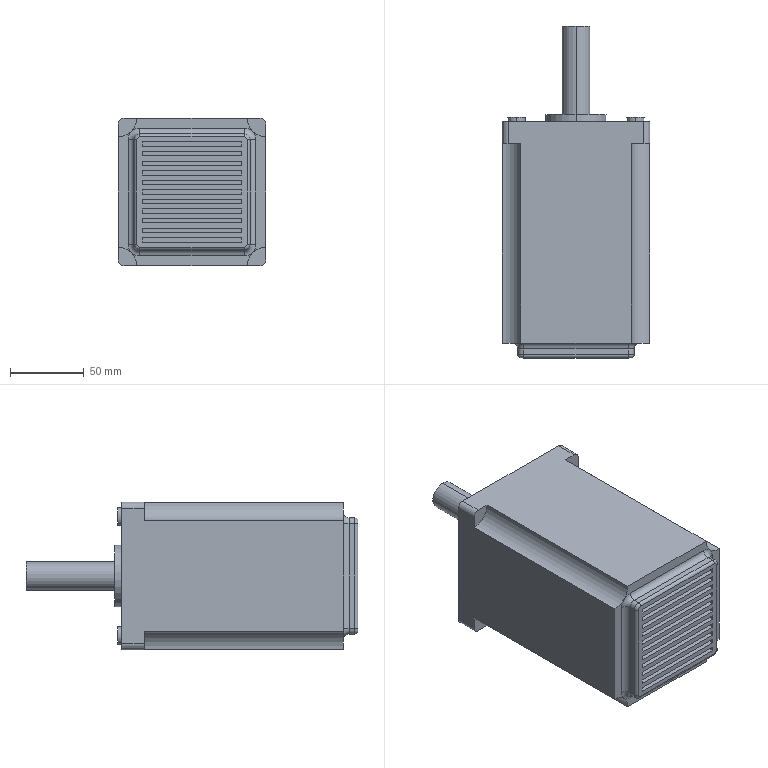Part | SolidWorks | features ICE 6, Fillet 3, CirPattern 1, Extrusion 1, LPattern 1 | 1 solid | 144 faces | box 100 x 225 x 100 mm | volume 1510650 mm3 | plane 104 | cylinder 32 | torus 8 | commonest cylinder face diameters 8 x12 12 x8 4 x4 25 x4 19 x2 41.585 x2